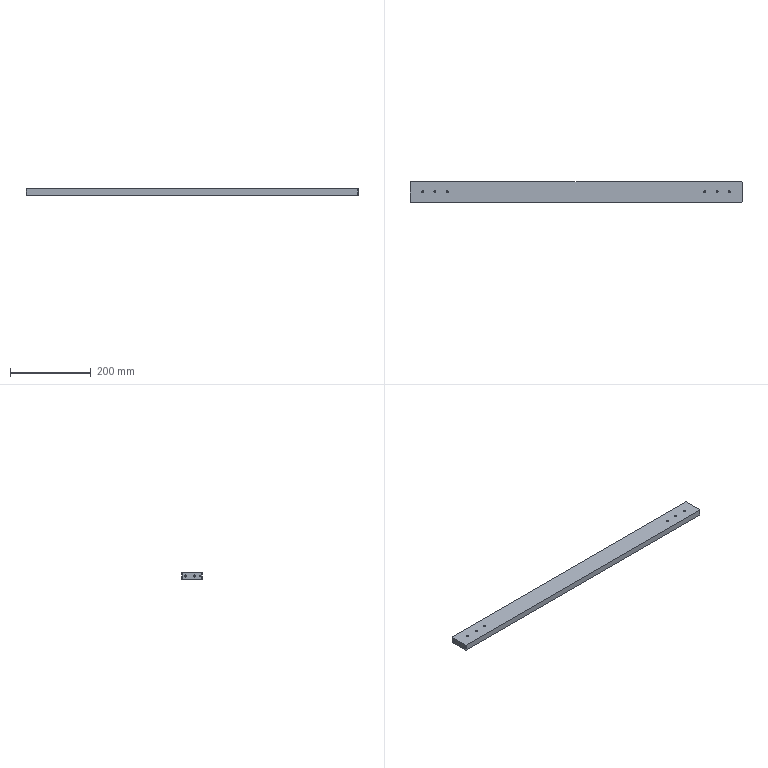Part | SolidWorks | features HoleWzd 3, Chamfer 1, Extrusion 1, MirrorPattern 1 | 1 solid | 46 faces | box 824 x 50 x 15 mm | volume 614536 mm3 | cylinder 24 | cone 12 | plane 10 | commonest cylinder face diameters 5 x20 3.3 x4
STEP:
#1=CARTESIAN_POINT('',(-29.5,25.,15.));
#2=VERTEX_POINT('',#1);
#3=CARTESIAN_POINT('',(-34.5,25.,15.));
#4=VERTEX_POINT('',#3);
#5=CARTESIAN_POINT('',(-32.,25.,15.));
#6=DIRECTION('',(0.,0.,-1.));
#7=DIRECTION('',(-1.,0.,0.));
#8=AXIS2_PLACEMENT_3D('',#5,#6,#7);
#9=CIRCLE('',#8,2.5);
#10=EDGE_CURVE('',#2,#4,#9,.T.);
#11=ORIENTED_EDGE('',*,*,#10,.F.);
#12=CARTESIAN_POINT('',(-29.5,25.,0.));
#13=VERTEX_POINT('',#12);
#14=CARTESIAN_POINT('',(-29.5,25.,0.));
#15=DIRECTION('',(0.,0.,-1.));
#16=VECTOR('',#15,1000.);
#17=LINE('',#14,#16);
#18=EDGE_CURVE('',#2,#13,#17,.T.);
#19=ORIENTED_EDGE('',*,*,#18,.T.);
#20=CARTESIAN_POINT('',(-34.5,25.,0.));
#21=VERTEX_POINT('',#20);
#22=CARTESIAN_POINT('',(-32.,25.,0.));
#23=DIRECTION('',(0.,0.,-1.));
#24=DIRECTION('',(-1.,0.,0.));
#25=AXIS2_PLACEMENT_3D('',#22,#23,#24);
#26=CIRCLE('',#25,2.5);
#27=EDGE_CURVE('',#13,#21,#26,.T.);
#28=ORIENTED_EDGE('',*,*,#27,.T.);
#29=CARTESIAN_POINT('',(-34.5,25.,0.));
#30=DIRECTION('',(0.,0.,-1.));
#31=VECTOR('',#30,1000.);
#32=LINE('',#29,#31);
#33=EDGE_CURVE('',#4,#21,#32,.T.);
#34=ORIENTED_EDGE('',*,*,#33,.F.);
#35=EDGE_LOOP('',(#11,#19,#28,#34));
#36=FACE_OUTER_BOUND('',#35,.T.);
#37=CARTESIAN_POINT('',(-32.,25.,0.));
#38=DIRECTION('',(0.,0.,-1.));
#39=DIRECTION('',(-1.,0.,0.));
#40=AXIS2_PLACEMENT_3D('',#37,#38,#39);
#41=CYLINDRICAL_SURFACE('',#40,2.5);
#42=ADVANCED_FACE('',(#36),#41,.F.);
#43=CARTESIAN_POINT('',(-59.5,25.,15.));
#44=VERTEX_POINT('',#43);
#45=CARTESIAN_POINT('',(-64.5,25.,15.));
#46=VERTEX_POINT('',#45);
#47=CARTESIAN_POINT('',(-62.,25.,15.));
#48=DIRECTION('',(0.,0.,-1.));
#49=DIRECTION('',(-1.,0.,0.));
#50=AXIS2_PLACEMENT_3D('',#47,#48,#49);
#51=CIRCLE('',#50,2.5);
#52=EDGE_CURVE('',#44,#46,#51,.T.);
#53=ORIENTED_EDGE('',*,*,#52,.F.);
#54=CARTESIAN_POINT('',(-59.5,25.,0.));
#55=VERTEX_POINT('',#54);
#56=CARTESIAN_POINT('',(-59.5,25.,0.));
#57=DIRECTION('',(0.,0.,-1.));
#58=VECTOR('',#57,1000.);
#59=LINE('',#56,#58);
#60=EDGE_CURVE('',#44,#55,#59,.T.);
#61=ORIENTED_EDGE('',*,*,#60,.T.);
#62=CARTESIAN_POINT('',(-64.5,25.,0.));
#63=VERTEX_POINT('',#62);
#64=CARTESIAN_POINT('',(-62.,25.,0.));
#65=DIRECTION('',(0.,0.,-1.));
#66=DIRECTION('',(-1.,0.,0.));
#67=AXIS2_PLACEMENT_3D('',#64,#65,#66);
#68=CIRCLE('',#67,2.5);
#69=EDGE_CURVE('',#55,#63,#68,.T.);
#70=ORIENTED_EDGE('',*,*,#69,.T.);
#71=CARTESIAN_POINT('',(-64.5,25.,0.));
#72=DIRECTION('',(0.,0.,-1.));
#73=VECTOR('',#72,1000.);
#74=LINE('',#71,#73);
#75=EDGE_CURVE('',#46,#63,#74,.T.);
#76=ORIENTED_EDGE('',*,*,#75,.F.);
#77=EDGE_LOOP('',(#53,#61,#70,#76));
#78=FACE_OUTER_BOUND('',#77,.T.);
#79=CARTESIAN_POINT('',(-62.,25.,0.));
#80=DIRECTION('',(0.,0.,-1.));
#81=DIRECTION('',(-1.,0.,0.));
#82=AXIS2_PLACEMENT_3D('',#79,#80,#81);
#83=CYLINDRICAL_SURFACE('',#82,2.5);
#84=ADVANCED_FACE('',(#78),#83,.F.);
#85=CARTESIAN_POINT('',(-89.5,25.,15.));
#86=VERTEX_POINT('',#85);
#87=CARTESIAN_POINT('',(-94.5,25.,15.));
#88=VERTEX_POINT('',#87);
#89=CARTESIAN_POINT('',(-92.,25.,15.));
#90=DIRECTION('',(0.,0.,-1.));
#91=DIRECTION('',(-1.,0.,0.));
#92=AXIS2_PLACEMENT_3D('',#89,#90,#91);
#93=CIRCLE('',#92,2.5);
#94=EDGE_CURVE('',#86,#88,#93,.T.);
#95=ORIENTED_EDGE('',*,*,#94,.F.);
#96=CARTESIAN_POINT('',(-89.5,25.,0.));
#97=VERTEX_POINT('',#96);
#98=CARTESIAN_POINT('',(-89.5,25.,0.));
#99=DIRECTION('',(0.,0.,-1.));
#100=VECTOR('',#99,1000.);
#101=LINE('',#98,#100);
#102=EDGE_CURVE('',#86,#97,#101,.T.);
#103=ORIENTED_EDGE('',*,*,#102,.T.);
#104=CARTESIAN_POINT('',(-94.5,25.,0.));
#105=VERTEX_POINT('',#104);
#106=CARTESIAN_POINT('',(-92.,25.,0.));
#107=DIRECTION('',(0.,0.,-1.));
#108=DIRECTION('',(-1.,0.,0.));
#109=AXIS2_PLACEMENT_3D('',#106,#107,#108);
#110=CIRCLE('',#109,2.5);
#111=EDGE_CURVE('',#97,#105,#110,.T.);
#112=ORIENTED_EDGE('',*,*,#111,.T.);
#113=CARTESIAN_POINT('',(-94.5,25.,0.));
#114=DIRECTION('',(0.,0.,-1.));
#115=VECTOR('',#114,1000.);
#116=LINE('',#113,#115);
#117=EDGE_CURVE('',#88,#105,#116,.T.);
#118=ORIENTED_EDGE('',*,*,#117,.F.);
#119=EDGE_LOOP('',(#95,#103,#112,#118));
#120=FACE_OUTER_BOUND('',#119,.T.);
#121=CARTESIAN_POINT('',(-92.,25.,0.));
#122=DIRECTION('',(0.,0.,-1.));
#123=DIRECTION('',(-1.,0.,0.));
#124=AXIS2_PLACEMENT_3D('',#121,#122,#123);
#125=CYLINDRICAL_SURFACE('',#124,2.5);
#126=ADVANCED_FACE('',(#120),#125,.F.);
#127=CARTESIAN_POINT('',(-729.5,25.,15.));
#128=VERTEX_POINT('',#127);
#129=CARTESIAN_POINT('',(-734.5,25.,15.));
#130=VERTEX_POINT('',#129);
#131=CARTESIAN_POINT('',(-732.,25.,15.));
#132=DIRECTION('',(0.,0.,-1.));
#133=DIRECTION('',(-1.,0.,0.));
#134=AXIS2_PLACEMENT_3D('',#131,#132,#133);
#135=CIRCLE('',#134,2.5);
#136=EDGE_CURVE('',#128,#130,#135,.T.);
#137=ORIENTED_EDGE('',*,*,#136,.F.);
#138=CARTESIAN_POINT('',(-729.5,25.,0.));
#139=VERTEX_POINT('',#138);
#140=CARTESIAN_POINT('',(-729.5,25.,0.));
#141=DIRECTION('',(0.,0.,-1.));
#142=VECTOR('',#141,1000.);
#143=LINE('',#140,#142);
#144=EDGE_CURVE('',#128,#139,#143,.T.);
#145=ORIENTED_EDGE('',*,*,#144,.T.);
#146=CARTESIAN_POINT('',(-734.5,25.,0.));
#147=VERTEX_POINT('',#146);
#148=CARTESIAN_POINT('',(-732.,25.,0.));
#149=DIRECTION('',(0.,0.,-1.));
#150=DIRECTION('',(-1.,0.,0.));
#151=AXIS2_PLACEMENT_3D('',#148,#149,#150);
#152=CIRCLE('',#151,2.5);
#153=EDGE_CURVE('',#139,#147,#152,.T.);
#154=ORIENTED_EDGE('',*,*,#153,.T.);
#155=CARTESIAN_POINT('',(-734.5,25.,0.));
#156=DIRECTION('',(0.,0.,-1.));
#157=VECTOR('',#156,1000.);
#158=LINE('',#155,#157);
#159=EDGE_CURVE('',#130,#147,#158,.T.);
#160=ORIENTED_EDGE('',*,*,#159,.F.);
#161=EDGE_LOOP('',(#137,#145,#154,#160));
#162=FACE_OUTER_BOUND('',#161,.T.);
#163=CARTESIAN_POINT('',(-732.,25.,0.));
#164=DIRECTION('',(0.,0.,-1.));
#165=DIRECTION('',(-1.,0.,0.));
#166=AXIS2_PLACEMENT_3D('',#163,#164,#165);
#167=CYLINDRICAL_SURFACE('',#166,2.5);
#168=ADVANCED_FACE('',(#162),#167,.F.);
#169=CARTESIAN_POINT('',(-759.5,25.,15.));
#170=VERTEX_POINT('',#169);
#171=CARTESIAN_POINT('',(-764.5,25.,15.));
#172=VERTEX_POINT('',#171);
#173=CARTESIAN_POINT('',(-762.,25.,15.));
#174=DIRECTION('',(0.,0.,-1.));
#175=DIRECTION('',(-1.,0.,0.));
#176=AXIS2_PLACEMENT_3D('',#173,#174,#175);
#177=CIRCLE('',#176,2.5);
#178=EDGE_CURVE('',#170,#172,#177,.T.);
#179=ORIENTED_EDGE('',*,*,#178,.F.);
#180=CARTESIAN_POINT('',(-759.5,25.,0.));
#181=VERTEX_POINT('',#180);
#182=CARTESIAN_POINT('',(-759.5,25.,0.));
#183=DIRECTION('',(0.,0.,-1.));
#184=VECTOR('',#183,1000.);
#185=LINE('',#182,#184);
#186=EDGE_CURVE('',#170,#181,#185,.T.);
#187=ORIENTED_EDGE('',*,*,#186,.T.);
#188=CARTESIAN_POINT('',(-764.5,25.,0.));
#189=VERTEX_POINT('',#188);
#190=CARTESIAN_POINT('',(-762.,25.,0.));
#191=DIRECTION('',(0.,0.,-1.));
#192=DIRECTION('',(-1.,0.,0.));
#193=AXIS2_PLACEMENT_3D('',#190,#191,#192);
#194=CIRCLE('',#193,2.5);
#195=EDGE_CURVE('',#181,#189,#194,.T.);
#196=ORIENTED_EDGE('',*,*,#195,.T.);
#197=CARTESIAN_POINT('',(-764.5,25.,0.));
#198=DIRECTION('',(0.,0.,-1.));
#199=VECTOR('',#198,1000.);
#200=LINE('',#197,#199);
#201=EDGE_CURVE('',#172,#189,#200,.T.);
#202=ORIENTED_EDGE('',*,*,#201,.F.);
#203=EDGE_LOOP('',(#179,#187,#196,#202));
#204=FACE_OUTER_BOUND('',#203,.T.);
#205=CARTESIAN_POINT('',(-762.,25.,0.));
#206=DIRECTION('',(0.,0.,-1.));
#207=DIRECTION('',(-1.,0.,0.));
#208=AXIS2_PLACEMENT_3D('',#205,#206,#207);
#209=CYLINDRICAL_SURFACE('',#208,2.5);
#210=ADVANCED_FACE('',(#204),#209,.F.);
#211=CARTESIAN_POINT('',(-789.5,25.,15.));
#212=VERTEX_POINT('',#211);
#213=CARTESIAN_POINT('',(-794.5,25.,15.));
#214=VERTEX_POINT('',#213);
#215=CARTESIAN_POINT('',(-792.,25.,15.));
#216=DIRECTION('',(0.,0.,-1.));
#217=DIRECTION('',(-1.,0.,0.));
#218=AXIS2_PLACEMENT_3D('',#215,#216,#217);
#219=CIRCLE('',#218,2.5);
#220=EDGE_CURVE('',#212,#214,#219,.T.);
#221=ORIENTED_EDGE('',*,*,#220,.F.);
#222=CARTESIAN_POINT('',(-789.5,25.,0.));
#223=VERTEX_POINT('',#222);
#224=CARTESIAN_POINT('',(-789.5,25.,0.));
#225=DIRECTION('',(0.,0.,-1.));
#226=VECTOR('',#225,1000.);
#227=LINE('',#224,#226);
#228=EDGE_CURVE('',#212,#223,#227,.T.);
#229=ORIENTED_EDGE('',*,*,#228,.T.);
#230=CARTESIAN_POINT('',(-794.5,25.,0.));
#231=VERTEX_POINT('',#230);
#232=CARTESIAN_POINT('',(-792.,25.,0.));
#233=DIRECTION('',(0.,0.,-1.));
#234=DIRECTION('',(-1.,0.,0.));
#235=AXIS2_PLACEMENT_3D('',#232,#233,#234);
#236=CIRCLE('',#235,2.5);
#237=EDGE_CURVE('',#223,#231,#236,.T.);
#238=ORIENTED_EDGE('',*,*,#237,.T.);
#239=CARTESIAN_POINT('',(-794.5,25.,0.));
#240=DIRECTION('',(0.,0.,-1.));
#241=VECTOR('',#240,1000.);
#242=LINE('',#239,#241);
#243=EDGE_CURVE('',#214,#231,#242,.T.);
#244=ORIENTED_EDGE('',*,*,#243,.F.);
#245=EDGE_LOOP('',(#221,#229,#238,#244));
#246=FACE_OUTER_BOUND('',#245,.T.);
#247=CARTESIAN_POINT('',(-792.,25.,0.));
#248=DIRECTION('',(0.,0.,-1.));
#249=DIRECTION('',(-1.,0.,0.));
#250=AXIS2_PLACEMENT_3D('',#247,#248,#249);
#251=CYLINDRICAL_SURFACE('',#250,2.5);
#252=ADVANCED_FACE('',(#246),#251,.F.);
#253=CARTESIAN_POINT('',(-812.5,5.,5.85));
#254=VERTEX_POINT('',#253);
#255=CARTESIAN_POINT('',(-812.5,5.,9.15));
#256=VERTEX_POINT('',#255);
#257=CARTESIAN_POINT('',(-812.5,5.,7.5));
#258=DIRECTION('',(-1.,0.,0.));
#259=DIRECTION('',(0.,0.,1.));
#260=AXIS2_PLACEMENT_3D('',#257,#258,#259);
#261=CIRCLE('',#260,1.65);
#262=EDGE_CURVE('',#254,#256,#261,.T.);
#263=ORIENTED_EDGE('',*,*,#262,.F.);
#264=CARTESIAN_POINT('',(-824.,5.,5.85));
#265=VERTEX_POINT('',#264);
#266=CARTESIAN_POINT('',(-824.,5.,5.85));
#267=DIRECTION('',(-1.,0.,0.));
#268=VECTOR('',#267,1000.);
#269=LINE('',#266,#268);
#270=EDGE_CURVE('',#254,#265,#269,.T.);
#271=ORIENTED_EDGE('',*,*,#270,.T.);
#272=CARTESIAN_POINT('',(-824.,5.,9.15));
#273=VERTEX_POINT('',#272);
#274=CARTESIAN_POINT('',(-824.,5.,7.5));
#275=DIRECTION('',(-1.,0.,0.));
#276=DIRECTION('',(0.,0.,1.));
#277=AXIS2_PLACEMENT_3D('',#274,#275,#276);
#278=CIRCLE('',#277,1.65);
#279=EDGE_CURVE('',#265,#273,#278,.T.);
#280=ORIENTED_EDGE('',*,*,#279,.T.);
#281=CARTESIAN_POINT('',(-824.,5.,9.15));
#282=DIRECTION('',(-1.,0.,0.));
#283=VECTOR('',#282,1000.);
#284=LINE('',#281,#283);
#285=EDGE_CURVE('',#256,#273,#284,.T.);
#286=ORIENTED_EDGE('',*,*,#285,.F.);
#287=EDGE_LOOP('',(#263,#271,#280,#286));
#288=FACE_OUTER_BOUND('',#287,.T.);
#289=CARTESIAN_POINT('',(-824.,5.,7.5));
#290=DIRECTION('',(-1.,0.,0.));
#291=DIRECTION('',(0.,0.,1.));
#292=AXIS2_PLACEMENT_3D('',#289,#290,#291);
#293=CYLINDRICAL_SURFACE('',#292,1.65);
#294=ADVANCED_FACE('',(#288),#293,.F.);
#295=CARTESIAN_POINT('',(-811.509,5.,7.5));
#296=VERTEX_POINT('',#295);
#297=CARTESIAN_POINT('',(-812.5,5.,9.15));
#298=DIRECTION('',(-0.515,0.,0.8572));
#299=VECTOR('',#298,1000.);
#300=LINE('',#297,#299);
#301=EDGE_CURVE('',#296,#256,#300,.T.);
#302=ORIENTED_EDGE('',*,*,#301,.F.);
#303=CARTESIAN_POINT('',(-812.5,5.,5.85));
#304=DIRECTION('',(-0.515,0.,-0.8572));
#305=VECTOR('',#304,1000.);
#306=LINE('',#303,#305);
#307=EDGE_CURVE('',#296,#254,#306,.T.);
#308=ORIENTED_EDGE('',*,*,#307,.T.);
#309=ORIENTED_EDGE('',*,*,#262,.T.);
#310=EDGE_LOOP('',(#302,#308,#309));
#311=FACE_OUTER_BOUND('',#310,.T.);
#312=CARTESIAN_POINT('',(-812.5,5.,7.5));
#313=DIRECTION('',(-1.,0.,0.));
#314=DIRECTION('',(0.,0.,1.));
#315=AXIS2_PLACEMENT_3D('',#312,#313,#314);
#316=CONICAL_SURFACE('',#315,1.65,1.03);
#317=ADVANCED_FACE('',(#311),#316,.F.);
#318=CARTESIAN_POINT('',(-807.,40.,5.));
#319=VERTEX_POINT('',#318);
#320=CARTESIAN_POINT('',(-807.,40.,10.));
#321=VERTEX_POINT('',#320);
#322=CARTESIAN_POINT('',(-807.,40.,7.5));
#323=DIRECTION('',(-1.,0.,0.));
#324=DIRECTION('',(0.,0.,1.));
#325=AXIS2_PLACEMENT_3D('',#322,#323,#324);
#326=CIRCLE('',#325,2.5);
#327=EDGE_CURVE('',#319,#321,#326,.T.);
#328=ORIENTED_EDGE('',*,*,#327,.F.);
#329=CARTESIAN_POINT('',(-824.,40.,5.));
#330=VERTEX_POINT('',#329);
#331=CARTESIAN_POINT('',(-824.,40.,5.));
#332=DIRECTION('',(-1.,0.,0.));
#333=VECTOR('',#332,1000.);
#334=LINE('',#331,#333);
#335=EDGE_CURVE('',#319,#330,#334,.T.);
#336=ORIENTED_EDGE('',*,*,#335,.T.);
#337=CARTESIAN_POINT('',(-824.,40.,10.));
#338=VERTEX_POINT('',#337);
#339=CARTESIAN_POINT('',(-824.,40.,7.5));
#340=DIRECTION('',(-1.,0.,0.));
#341=DIRECTION('',(0.,0.,1.));
#342=AXIS2_PLACEMENT_3D('',#339,#340,#341);
#343=CIRCLE('',#342,2.5);
#344=EDGE_CURVE('',#330,#338,#343,.T.);
#345=ORIENTED_EDGE('',*,*,#344,.T.);
#346=CARTESIAN_POINT('',(-824.,40.,10.));
#347=DIRECTION('',(-1.,0.,0.));
#348=VECTOR('',#347,1000.);
#349=LINE('',#346,#348);
#350=EDGE_CURVE('',#321,#338,#349,.T.);
#351=ORIENTED_EDGE('',*,*,#350,.F.);
#352=EDGE_LOOP('',(#328,#336,#345,#351));
#353=FACE_OUTER_BOUND('',#352,.T.);
#354=CARTESIAN_POINT('',(-824.,40.,7.5));
#355=DIRECTION('',(-1.,0.,0.));
#356=DIRECTION('',(0.,0.,1.));
#357=AXIS2_PLACEMENT_3D('',#354,#355,#356);
#358=CYLINDRICAL_SURFACE('',#357,2.5);
#359=ADVANCED_FACE('',(#353),#358,.F.);
#360=CARTESIAN_POINT('',(-805.498,40.,7.5));
#361=VERTEX_POINT('',#360);
#362=CARTESIAN_POINT('',(-807.,40.,10.));
#363=DIRECTION('',(-0.515,0.,0.8572));
#364=VECTOR('',#363,1000.);
#365=LINE('',#362,#364);
#366=EDGE_CURVE('',#361,#321,#365,.T.);
#367=ORIENTED_EDGE('',*,*,#366,.F.);
#368=CARTESIAN_POINT('',(-807.,40.,5.));
#369=DIRECTION('',(-0.515,0.,-0.8572));
#370=VECTOR('',#369,1000.);
#371=LINE('',#368,#370);
#372=EDGE_CURVE('',#361,#319,#371,.T.);
#373=ORIENTED_EDGE('',*,*,#372,.T.);
#374=ORIENTED_EDGE('',*,*,#327,.T.);
#375=EDGE_LOOP('',(#367,#373,#374));
#376=FACE_OUTER_BOUND('',#375,.T.);
#377=CARTESIAN_POINT('',(-807.,40.,7.5));
#378=DIRECTION('',(-1.,0.,0.));
#379=DIRECTION('',(0.,0.,1.));
#380=AXIS2_PLACEMENT_3D('',#377,#378,#379);
#381=CONICAL_SURFACE('',#380,2.5,1.03);
#382=ADVANCED_FACE('',(#376),#381,.F.);
#383=CARTESIAN_POINT('',(-807.,20.,5.));
#384=VERTEX_POINT('',#383);
#385=CARTESIAN_POINT('',(-807.,20.,10.));
#386=VERTEX_POINT('',#385);
#387=CARTESIAN_POINT('',(-807.,20.,7.5));
#388=DIRECTION('',(-1.,0.,0.));
#389=DIRECTION('',(0.,0.,1.));
#390=AXIS2_PLACEMENT_3D('',#387,#388,#389);
#391=CIRCLE('',#390,2.5);
#392=EDGE_CURVE('',#384,#386,#391,.T.);
#393=ORIENTED_EDGE('',*,*,#392,.F.);
#394=CARTESIAN_POINT('',(-824.,20.,5.));
#395=VERTEX_POINT('',#394);
#396=CARTESIAN_POINT('',(-824.,20.,5.));
#397=DIRECTION('',(-1.,0.,0.));
#398=VECTOR('',#397,1000.);
#399=LINE('',#396,#398);
#400=EDGE_CURVE('',#384,#395,#399,.T.);
#401=ORIENTED_EDGE('',*,*,#400,.T.);
#402=CARTESIAN_POINT('',(-824.,20.,10.));
#403=VERTEX_POINT('',#402);
#404=CARTESIAN_POINT('',(-824.,20.,7.5));
#405=DIRECTION('',(-1.,0.,0.));
#406=DIRECTION('',(0.,0.,1.));
#407=AXIS2_PLACEMENT_3D('',#404,#405,#406);
#408=CIRCLE('',#407,2.5);
#409=EDGE_CURVE('',#395,#403,#408,.T.);
#410=ORIENTED_EDGE('',*,*,#409,.T.);
#411=CARTESIAN_POINT('',(-824.,20.,10.));
#412=DIRECTION('',(-1.,0.,0.));
#413=VECTOR('',#412,1000.);
#414=LINE('',#411,#413);
#415=EDGE_CURVE('',#386,#403,#414,.T.);
#416=ORIENTED_EDGE('',*,*,#415,.F.);
#417=EDGE_LOOP('',(#393,#401,#410,#416));
#418=FACE_OUTER_BOUND('',#417,.T.);
#419=CARTESIAN_POINT('',(-824.,20.,7.5));
#420=DIRECTION('',(-1.,0.,0.));
#421=DIRECTION('',(0.,0.,1.));
#422=AXIS2_PLACEMENT_3D('',#419,#420,#421);
#423=CYLINDRICAL_SURFACE('',#422,2.5);
#424=ADVANCED_FACE('',(#418),#423,.F.);
#425=CARTESIAN_POINT('',(-805.498,20.,7.5));
#426=VERTEX_POINT('',#425);
#427=CARTESIAN_POINT('',(-807.,20.,10.));
#428=DIRECTION('',(-0.515,0.,0.8572));
#429=VECTOR('',#428,1000.);
#430=LINE('',#427,#429);
#431=EDGE_CURVE('',#426,#386,#430,.T.);
#432=ORIENTED_EDGE('',*,*,#431,.F.);
#433=CARTESIAN_POINT('',(-807.,20.,5.));
#434=DIRECTION('',(-0.515,0.,-0.8572));
#435=VECTOR('',#434,1000.);
#436=LINE('',#433,#435);
#437=EDGE_CURVE('',#426,#384,#436,.T.);
#438=ORIENTED_EDGE('',*,*,#437,.T.);
#439=ORIENTED_EDGE('',*,*,#392,.T.);
#440=EDGE_LOOP('',(#432,#438,#439));
#441=FACE_OUTER_BOUND('',#440,.T.);
#442=CARTESIAN_POINT('',(-807.,20.,7.5));
#443=DIRECTION('',(-1.,0.,0.));
#444=DIRECTION('',(0.,0.,1.));
#445=AXIS2_PLACEMENT_3D('',#442,#443,#444);
#446=CONICAL_SURFACE('',#445,2.5,1.03);
#447=ADVANCED_FACE('',(#441),#446,.F.);
#448=CARTESIAN_POINT('',(-11.5,5.,9.15));
#449=VERTEX_POINT('',#448);
#450=CARTESIAN_POINT('',(-11.5,5.,5.85));
#451=VERTEX_POINT('',#450);
#452=CARTESIAN_POINT('',(-11.5,5.,7.5));
#453=DIRECTION('',(1.,0.,0.));
#454=DIRECTION('',(0.,0.,-1.));
#455=AXIS2_PLACEMENT_3D('',#452,#453,#454);
#456=CIRCLE('',#455,1.65);
#457=EDGE_CURVE('',#449,#451,#456,.T.);
#458=ORIENTED_EDGE('',*,*,#457,.F.);
#459=CARTESIAN_POINT('',(0.,5.,9.15));
#460=VERTEX_POINT('',#459);
#461=CARTESIAN_POINT('',(0.,5.,9.15));
#462=DIRECTION('',(1.,0.,0.));
#463=VECTOR('',#462,1000.);
#464=LINE('',#461,#463);
#465=EDGE_CURVE('',#449,#460,#464,.T.);
#466=ORIENTED_EDGE('',*,*,#465,.T.);
#467=CARTESIAN_POINT('',(0.,5.,5.85));
#468=VERTEX_POINT('',#467);
#469=CARTESIAN_POINT('',(0.,5.,7.5));
#470=DIRECTION('',(1.,0.,0.));
#471=DIRECTION('',(0.,0.,-1.));
#472=AXIS2_PLACEMENT_3D('',#469,#470,#471);
#473=CIRCLE('',#472,1.65);
#474=EDGE_CURVE('',#460,#468,#473,.T.);
#475=ORIENTED_EDGE('',*,*,#474,.T.);
#476=CARTESIAN_POINT('',(0.,5.,5.85));
#477=DIRECTION('',(1.,0.,0.));
#478=VECTOR('',#477,1000.);
#479=LINE('',#476,#478);
#480=EDGE_CURVE('',#451,#468,#479,.T.);
#481=ORIENTED_EDGE('',*,*,#480,.F.);
#482=EDGE_LOOP('',(#458,#466,#475,#481));
#483=FACE_OUTER_BOUND('',#482,.T.);
#484=CARTESIAN_POINT('',(0.,5.,7.5));
#485=DIRECTION('',(1.,0.,0.));
#486=DIRECTION('',(0.,0.,-1.));
#487=AXIS2_PLACEMENT_3D('',#484,#485,#486);
#488=CYLINDRICAL_SURFACE('',#487,1.65);
#489=ADVANCED_FACE('',(#483),#488,.F.);
#490=CARTESIAN_POINT('',(-12.491,5.,7.5));
#491=VERTEX_POINT('',#490);
#492=CARTESIAN_POINT('',(-11.5,5.,5.85));
#493=DIRECTION('',(0.515,0.,-0.8572));
#494=VECTOR('',#493,1000.);
#495=LINE('',#492,#494);
#496=EDGE_CURVE('',#491,#451,#495,.T.);
#497=ORIENTED_EDGE('',*,*,#496,.F.);
#498=CARTESIAN_POINT('',(-11.5,5.,9.15));
#499=DIRECTION('',(0.515,0.,0.8572));
#500=VECTOR('',#499,1000.);
#501=LINE('',#498,#500);
#502=EDGE_CURVE('',#491,#449,#501,.T.);
#503=ORIENTED_EDGE('',*,*,#502,.T.);
#504=ORIENTED_EDGE('',*,*,#457,.T.);
#505=EDGE_LOOP('',(#497,#503,#504));
#506=FACE_OUTER_BOUND('',#505,.T.);
#507=CARTESIAN_POINT('',(-11.5,5.,7.5));
#508=DIRECTION('',(1.,0.,0.));
#509=DIRECTION('',(0.,0.,-1.));
#510=AXIS2_PLACEMENT_3D('',#507,#508,#509);
#511=CONICAL_SURFACE('',#510,1.65,1.03);
#512=ADVANCED_FACE('',(#506),#511,.F.);
#513=CARTESIAN_POINT('',(-17.,40.,10.));
#514=VERTEX_POINT('',#513);
#515=CARTESIAN_POINT('',(-17.,40.,5.));
#516=VERTEX_POINT('',#515);
#517=CARTESIAN_POINT('',(-17.,40.,7.5));
#518=DIRECTION('',(1.,0.,0.));
#519=DIRECTION('',(0.,0.,-1.));
#520=AXIS2_PLACEMENT_3D('',#517,#518,#519);
#521=CIRCLE('',#520,2.5);
#522=EDGE_CURVE('',#514,#516,#521,.T.);
#523=ORIENTED_EDGE('',*,*,#522,.F.);
#524=CARTESIAN_POINT('',(0.,40.,10.));
#525=VERTEX_POINT('',#524);
#526=CARTESIAN_POINT('',(0.,40.,10.));
#527=DIRECTION('',(1.,0.,0.));
#528=VECTOR('',#527,1000.);
#529=LINE('',#526,#528);
#530=EDGE_CURVE('',#514,#525,#529,.T.);
#531=ORIENTED_EDGE('',*,*,#530,.T.);
#532=CARTESIAN_POINT('',(0.,40.,5.));
#533=VERTEX_POINT('',#532);
#534=CARTESIAN_POINT('',(0.,40.,7.5));
#535=DIRECTION('',(1.,0.,0.));
#536=DIRECTION('',(0.,0.,-1.));
#537=AXIS2_PLACEMENT_3D('',#534,#535,#536);
#538=CIRCLE('',#537,2.5);
#539=EDGE_CURVE('',#525,#533,#538,.T.);
#540=ORIENTED_EDGE('',*,*,#539,.T.);
#541=CARTESIAN_POINT('',(0.,40.,5.));
#542=DIRECTION('',(1.,0.,0.));
#543=VECTOR('',#542,1000.);
#544=LINE('',#541,#543);
#545=EDGE_CURVE('',#516,#533,#544,.T.);
#546=ORIENTED_EDGE('',*,*,#545,.F.);
#547=EDGE_LOOP('',(#523,#531,#540,#546));
#548=FACE_OUTER_BOUND('',#547,.T.);
#549=CARTESIAN_POINT('',(0.,40.,7.5));
#550=DIRECTION('',(1.,0.,0.));
#551=DIRECTION('',(0.,0.,-1.));
#552=AXIS2_PLACEMENT_3D('',#549,#550,#551);
#553=CYLINDRICAL_SURFACE('',#552,2.5);
#554=ADVANCED_FACE('',(#548),#553,.F.);
#555=CARTESIAN_POINT('',(-18.502,40.,7.5));
#556=VERTEX_POINT('',#555);
#557=CARTESIAN_POINT('',(-17.,40.,5.));
#558=DIRECTION('',(0.515,0.,-0.8572));
#559=VECTOR('',#558,1000.);
#560=LINE('',#557,#559);
#561=EDGE_CURVE('',#556,#516,#560,.T.);
#562=ORIENTED_EDGE('',*,*,#561,.F.);
#563=CARTESIAN_POINT('',(-17.,40.,10.));
#564=DIRECTION('',(0.515,0.,0.8572));
#565=VECTOR('',#564,1000.);
#566=LINE('',#563,#565);
#567=EDGE_CURVE('',#556,#514,#566,.T.);
#568=ORIENTED_EDGE('',*,*,#567,.T.);
#569=ORIENTED_EDGE('',*,*,#522,.T.);
#570=EDGE_LOOP('',(#562,#568,#569));
#571=FACE_OUTER_BOUND('',#570,.T.);
#572=CARTESIAN_POINT('',(-17.,40.,7.5));
#573=DIRECTION('',(1.,0.,0.));
#574=DIRECTION('',(0.,0.,-1.));
#575=AXIS2_PLACEMENT_3D('',#572,#573,#574);
#576=CONICAL_SURFACE('',#575,2.5,1.03);
#577=ADVANCED_FACE('',(#571),#576,.F.);
#578=CARTESIAN_POINT('',(-17.,20.,10.));
#579=VERTEX_POINT('',#578);
#580=CARTESIAN_POINT('',(-17.,20.,5.));
#581=VERTEX_POINT('',#580);
#582=CARTESIAN_POINT('',(-17.,20.,7.5));
#583=DIRECTION('',(1.,0.,0.));
#584=DIRECTION('',(0.,0.,-1.));
#585=AXIS2_PLACEMENT_3D('',#582,#583,#584);
#586=CIRCLE('',#585,2.5);
#587=EDGE_CURVE('',#579,#581,#586,.T.);
#588=ORIENTED_EDGE('',*,*,#587,.F.);
#589=CARTESIAN_POINT('',(0.,20.,10.));
#590=VERTEX_POINT('',#589);
#591=CARTESIAN_POINT('',(0.,20.,10.));
#592=DIRECTION('',(1.,0.,0.));
#593=VECTOR('',#592,1000.);
#594=LINE('',#591,#593);
#595=EDGE_CURVE('',#579,#590,#594,.T.);
#596=ORIENTED_EDGE('',*,*,#595,.T.);
#597=CARTESIAN_POINT('',(0.,20.,5.));
#598=VERTEX_POINT('',#597);
#599=CARTESIAN_POINT('',(0.,20.,7.5));
#600=DIRECTION('',(1.,0.,0.));
#601=DIRECTION('',(0.,0.,-1.));
#602=AXIS2_PLACEMENT_3D('',#599,#600,#601);
#603=CIRCLE('',#602,2.5);
#604=EDGE_CURVE('',#590,#598,#603,.T.);
#605=ORIENTED_EDGE('',*,*,#604,.T.);
#606=CARTESIAN_POINT('',(0.,20.,5.));
#607=DIRECTION('',(1.,0.,0.));
#608=VECTOR('',#607,1000.);
#609=LINE('',#606,#608);
#610=EDGE_CURVE('',#581,#598,#609,.T.);
#611=ORIENTED_EDGE('',*,*,#610,.F.);
#612=EDGE_LOOP('',(#588,#596,#605,#611));
#613=FACE_OUTER_BOUND('',#612,.T.);
#614=CARTESIAN_POINT('',(0.,20.,7.5));
#615=DIRECTION('',(1.,0.,0.));
#616=DIRECTION('',(0.,0.,-1.));
#617=AXIS2_PLACEMENT_3D('',#614,#615,#616);
#618=CYLINDRICAL_SURFACE('',#617,2.5);
#619=ADVANCED_FACE('',(#613),#618,.F.);
#620=CARTESIAN_POINT('',(-18.502,20.,7.5));
#621=VERTEX_POINT('',#620);
#622=CARTESIAN_POINT('',(-17.,20.,5.));
#623=DIRECTION('',(0.515,0.,-0.8572));
#624=VECTOR('',#623,1000.);
#625=LINE('',#622,#624);
#626=EDGE_CURVE('',#621,#581,#625,.T.);
#627=ORIENTED_EDGE('',*,*,#626,.F.);
#628=CARTESIAN_POINT('',(-17.,20.,10.));
#629=DIRECTION('',(0.515,0.,0.8572));
#630=VECTOR('',#629,1000.);
#631=LINE('',#628,#630);
#632=EDGE_CURVE('',#621,#579,#631,.T.);
#633=ORIENTED_EDGE('',*,*,#632,.T.);
#634=ORIENTED_EDGE('',*,*,#587,.T.);
#635=EDGE_LOOP('',(#627,#633,#634));
#636=FACE_OUTER_BOUND('',#635,.T.);
#637=CARTESIAN_POINT('',(-17.,20.,7.5));
#638=DIRECTION('',(1.,0.,0.));
#639=DIRECTION('',(0.,0.,-1.));
#640=AXIS2_PLACEMENT_3D('',#637,#638,#639);
#641=CONICAL_SURFACE('',#640,2.5,1.03);
#642=ADVANCED_FACE('',(#636),#641,.F.);
#643=CARTESIAN_POINT('',(-2.,50.,0.));
#644=VERTEX_POINT('',#643);
#645=CARTESIAN_POINT('',(-822.,50.,0.));
#646=VERTEX_POINT('',#645);
#647=CARTESIAN_POINT('',(-824.,50.,0.));
#648=DIRECTION('',(-1.,0.,0.));
#649=VECTOR('',#648,1000.);
#650=LINE('',#647,#649);
#651=EDGE_CURVE('',#644,#646,#650,.T.);
#652=ORIENTED_EDGE('',*,*,#651,.T.);
#653=CARTESIAN_POINT('',(-822.,50.,15.));
#654=VERTEX_POINT('',#653);
#655=CARTESIAN_POINT('',(-822.,50.,15.));
#656=DIRECTION('',(0.,0.,1.));
#657=VECTOR('',#656,1000.);
#658=LINE('',#655,#657);
#659=EDGE_CURVE('',#646,#654,#658,.T.);
#660=ORIENTED_EDGE('',*,*,#659,.T.);
#661=CARTESIAN_POINT('',(-2.,50.,15.));
#662=VERTEX_POINT('',#661);
#663=CARTESIAN_POINT('',(-824.,50.,15.));
#664=DIRECTION('',(-1.,0.,0.));
#665=VECTOR('',#664,1000.);
#666=LINE('',#663,#665);
#667=EDGE_CURVE('',#662,#654,#666,.T.);
#668=ORIENTED_EDGE('',*,*,#667,.F.);
#669=CARTESIAN_POINT('',(-2.,50.,15.));
#670=DIRECTION('',(0.,0.,-1.));
#671=VECTOR('',#670,1000.);
#672=LINE('',#669,#671);
#673=EDGE_CURVE('',#662,#644,#672,.T.);
#674=ORIENTED_EDGE('',*,*,#673,.T.);
#675=EDGE_LOOP('',(#652,#660,#668,#674));
#676=FACE_OUTER_BOUND('',#675,.T.);
#677=CARTESIAN_POINT('',(-824.,50.,15.));
#678=DIRECTION('',(0.,-1.,0.));
#679=DIRECTION('',(1.,0.,0.));
#680=AXIS2_PLACEMENT_3D('',#677,#678,#679);
#681=PLANE('',#680);
#682=ADVANCED_FACE('',(#676),#681,.F.);
#683=CARTESIAN_POINT('',(-824.,5.,7.5));
#684=DIRECTION('',(-1.,0.,0.));
#685=DIRECTION('',(0.,0.,1.));
#686=AXIS2_PLACEMENT_3D('',#683,#684,#685);
#687=CIRCLE('',#686,1.65);
#688=EDGE_CURVE('',#273,#265,#687,.T.);
#689=ORIENTED_EDGE('',*,*,#688,.F.);
#690=ORIENTED_EDGE('',*,*,#279,.F.);
#691=EDGE_LOOP('',(#689,#690));
#692=FACE_BOUND('',#691,.T.);
#693=CARTESIAN_POINT('',(-824.,40.,7.5));
#694=DIRECTION('',(-1.,0.,0.));
#695=DIRECTION('',(0.,0.,1.));
#696=AXIS2_PLACEMENT_3D('',#693,#694,#695);
#697=CIRCLE('',#696,2.5);
#698=EDGE_CURVE('',#338,#330,#697,.T.);
#699=ORIENTED_EDGE('',*,*,#698,.F.);
#700=ORIENTED_EDGE('',*,*,#344,.F.);
#701=EDGE_LOOP('',(#699,#700));
#702=FACE_BOUND('',#701,.T.);
#703=CARTESIAN_POINT('',(-824.,20.,7.5));
#704=DIRECTION('',(-1.,0.,0.));
#705=DIRECTION('',(0.,0.,1.));
#706=AXIS2_PLACEMENT_3D('',#703,#704,#705);
#707=CIRCLE('',#706,2.5);
#708=EDGE_CURVE('',#403,#395,#707,.T.);
#709=ORIENTED_EDGE('',*,*,#708,.F.);
#710=ORIENTED_EDGE('',*,*,#409,.F.);
#711=EDGE_LOOP('',(#709,#710));
#712=FACE_BOUND('',#711,.T.);
#713=CARTESIAN_POINT('',(-824.,48.,15.));
#714=VERTEX_POINT('',#713);
#715=CARTESIAN_POINT('',(-824.,2.,15.));
#716=VERTEX_POINT('',#715);
#717=CARTESIAN_POINT('',(-824.,50.,15.));
#718=DIRECTION('',(0.,-1.,0.));
#719=VECTOR('',#718,1000.);
#720=LINE('',#717,#719);
#721=EDGE_CURVE('',#714,#716,#720,.T.);
#722=ORIENTED_EDGE('',*,*,#721,.F.);
#723=CARTESIAN_POINT('',(-824.,48.,0.));
#724=VERTEX_POINT('',#723);
#725=CARTESIAN_POINT('',(-824.,48.,15.));
#726=DIRECTION('',(0.,0.,-1.));
#727=VECTOR('',#726,1000.);
#728=LINE('',#725,#727);
#729=EDGE_CURVE('',#714,#724,#728,.T.);
#730=ORIENTED_EDGE('',*,*,#729,.T.);
#731=CARTESIAN_POINT('',(-824.,2.,0.));
#732=VERTEX_POINT('',#731);
#733=CARTESIAN_POINT('',(-824.,50.,0.));
#734=DIRECTION('',(0.,-1.,0.));
#735=VECTOR('',#734,1000.);
#736=LINE('',#733,#735);
#737=EDGE_CURVE('',#724,#732,#736,.T.);
#738=ORIENTED_EDGE('',*,*,#737,.T.);
#739=CARTESIAN_POINT('',(-824.,2.,15.));
#740=DIRECTION('',(0.,0.,1.));
#741=VECTOR('',#740,1000.);
#742=LINE('',#739,#741);
#743=EDGE_CURVE('',#732,#716,#742,.T.);
#744=ORIENTED_EDGE('',*,*,#743,.T.);
#745=EDGE_LOOP('',(#722,#730,#738,#744));
#746=FACE_OUTER_BOUND('',#745,.T.);
#747=CARTESIAN_POINT('',(-824.,50.,15.));
#748=DIRECTION('',(1.,0.,0.));
#749=DIRECTION('',(0.,1.,0.));
#750=AXIS2_PLACEMENT_3D('',#747,#748,#749);
#751=PLANE('',#750);
#752=ADVANCED_FACE('',(#692,#702,#712,#746),#751,.F.);
#753=CARTESIAN_POINT('',(-822.,0.,15.));
#754=VERTEX_POINT('',#753);
#755=CARTESIAN_POINT('',(-2.,0.,15.));
#756=VERTEX_POINT('',#755);
#757=CARTESIAN_POINT('',(-824.,0.,15.));
#758=DIRECTION('',(1.,0.,0.));
#759=VECTOR('',#758,1000.);
#760=LINE('',#757,#759);
#761=EDGE_CURVE('',#754,#756,#760,.T.);
#762=ORIENTED_EDGE('',*,*,#761,.F.);
#763=CARTESIAN_POINT('',(-822.,0.,0.));
#764=VERTEX_POINT('',#763);
#765=CARTESIAN_POINT('',(-822.,0.,15.));
#766=DIRECTION('',(0.,0.,-1.));
#767=VECTOR('',#766,1000.);
#768=LINE('',#765,#767);
#769=EDGE_CURVE('',#754,#764,#768,.T.);
#770=ORIENTED_EDGE('',*,*,#769,.T.);
#771=CARTESIAN_POINT('',(-2.,0.,0.));
#772=VERTEX_POINT('',#771);
#773=CARTESIAN_POINT('',(-824.,0.,0.));
#774=DIRECTION('',(1.,0.,0.));
#775=VECTOR('',#774,1000.);
#776=LINE('',#773,#775);
#777=EDGE_CURVE('',#764,#772,#776,.T.);
#778=ORIENTED_EDGE('',*,*,#777,.T.);
#779=CARTESIAN_POINT('',(-2.,0.,15.));
#780=DIRECTION('',(0.,0.,1.));
#781=VECTOR('',#780,1000.);
#782=LINE('',#779,#781);
#783=EDGE_CURVE('',#772,#756,#782,.T.);
#784=ORIENTED_EDGE('',*,*,#783,.T.);
#785=EDGE_LOOP('',(#762,#770,#778,#784));
#786=FACE_OUTER_BOUND('',#785,.T.);
#787=CARTESIAN_POINT('',(-824.,0.,15.));
#788=DIRECTION('',(0.,1.,0.));
#789=DIRECTION('',(0.,0.,1.));
#790=AXIS2_PLACEMENT_3D('',#787,#788,#789);
#791=PLANE('',#790);
#792=ADVANCED_FACE('',(#786),#791,.F.);
#793=CARTESIAN_POINT('',(0.,5.,7.5));
#794=DIRECTION('',(1.,0.,0.));
#795=DIRECTION('',(0.,0.,-1.));
#796=AXIS2_PLACEMENT_3D('',#793,#794,#795);
#797=CIRCLE('',#796,1.65);
#798=EDGE_CURVE('',#468,#460,#797,.T.);
#799=ORIENTED_EDGE('',*,*,#798,.F.);
#800=ORIENTED_EDGE('',*,*,#474,.F.);
#801=EDGE_LOOP('',(#799,#800));
#802=FACE_BOUND('',#801,.T.);
#803=CARTESIAN_POINT('',(0.,40.,7.5));
#804=DIRECTION('',(1.,0.,0.));
#805=DIRECTION('',(0.,0.,-1.));
#806=AXIS2_PLACEMENT_3D('',#803,#804,#805);
#807=CIRCLE('',#806,2.5);
#808=EDGE_CURVE('',#533,#525,#807,.T.);
#809=ORIENTED_EDGE('',*,*,#808,.F.);
#810=ORIENTED_EDGE('',*,*,#539,.F.);
#811=EDGE_LOOP('',(#809,#810));
#812=FACE_BOUND('',#811,.T.);
#813=CARTESIAN_POINT('',(0.,20.,7.5));
#814=DIRECTION('',(1.,0.,0.));
#815=DIRECTION('',(0.,0.,-1.));
#816=AXIS2_PLACEMENT_3D('',#813,#814,#815);
#817=CIRCLE('',#816,2.5);
#818=EDGE_CURVE('',#598,#590,#817,.T.);
#819=ORIENTED_EDGE('',*,*,#818,.F.);
#820=ORIENTED_EDGE('',*,*,#604,.F.);
#821=EDGE_LOOP('',(#819,#820));
#822=FACE_BOUND('',#821,.T.);
#823=CARTESIAN_POINT('',(0.,2.,0.));
#824=VERTEX_POINT('',#823);
#825=CARTESIAN_POINT('',(0.,48.,0.));
#826=VERTEX_POINT('',#825);
#827=CARTESIAN_POINT('',(0.,50.,0.));
#828=DIRECTION('',(0.,1.,0.));
#829=VECTOR('',#828,1000.);
#830=LINE('',#827,#829);
#831=EDGE_CURVE('',#824,#826,#830,.T.);
#832=ORIENTED_EDGE('',*,*,#831,.T.);
#833=CARTESIAN_POINT('',(0.,48.,15.));
#834=VERTEX_POINT('',#833);
#835=CARTESIAN_POINT('',(0.,48.,15.));
#836=DIRECTION('',(0.,0.,1.));
#837=VECTOR('',#836,1000.);
#838=LINE('',#835,#837);
#839=EDGE_CURVE('',#826,#834,#838,.T.);
#840=ORIENTED_EDGE('',*,*,#839,.T.);
#841=CARTESIAN_POINT('',(0.,2.,15.));
#842=VERTEX_POINT('',#841);
#843=CARTESIAN_POINT('',(0.,50.,15.));
#844=DIRECTION('',(0.,1.,0.));
#845=VECTOR('',#844,1000.);
#846=LINE('',#843,#845);
#847=EDGE_CURVE('',#842,#834,#846,.T.);
#848=ORIENTED_EDGE('',*,*,#847,.F.);
#849=CARTESIAN_POINT('',(0.,2.,15.));
#850=DIRECTION('',(0.,0.,-1.));
#851=VECTOR('',#850,1000.);
#852=LINE('',#849,#851);
#853=EDGE_CURVE('',#842,#824,#852,.T.);
#854=ORIENTED_EDGE('',*,*,#853,.T.);
#855=EDGE_LOOP('',(#832,#840,#848,#854));
#856=FACE_OUTER_BOUND('',#855,.T.);
#857=CARTESIAN_POINT('',(0.,50.,15.));
#858=DIRECTION('',(-1.,0.,0.));
#859=DIRECTION('',(0.,-1.,0.));
#860=AXIS2_PLACEMENT_3D('',#857,#858,#859);
#861=PLANE('',#860);
#862=ADVANCED_FACE('',(#802,#812,#822,#856),#861,.F.);
#863=CARTESIAN_POINT('',(-32.,25.,15.));
#864=DIRECTION('',(0.,0.,-1.));
#865=DIRECTION('',(-1.,0.,0.));
#866=AXIS2_PLACEMENT_3D('',#863,#864,#865);
#867=CIRCLE('',#866,2.5);
#868=EDGE_CURVE('',#4,#2,#867,.T.);
#869=ORIENTED_EDGE('',*,*,#868,.T.);
#870=ORIENTED_EDGE('',*,*,#10,.T.);
#871=EDGE_LOOP('',(#869,#870));
#872=FACE_BOUND('',#871,.T.);
#873=CARTESIAN_POINT('',(-62.,25.,15.));
#874=DIRECTION('',(0.,0.,-1.));
#875=DIRECTION('',(-1.,0.,0.));
#876=AXIS2_PLACEMENT_3D('',#873,#874,#875);
#877=CIRCLE('',#876,2.5);
#878=EDGE_CURVE('',#46,#44,#877,.T.);
#879=ORIENTED_EDGE('',*,*,#878,.T.);
#880=ORIENTED_EDGE('',*,*,#52,.T.);
#881=EDGE_LOOP('',(#879,#880));
#882=FACE_BOUND('',#881,.T.);
#883=CARTESIAN_POINT('',(-92.,25.,15.));
#884=DIRECTION('',(0.,0.,-1.));
#885=DIRECTION('',(-1.,0.,0.));
#886=AXIS2_PLACEMENT_3D('',#883,#884,#885);
#887=CIRCLE('',#886,2.5);
#888=EDGE_CURVE('',#88,#86,#887,.T.);
#889=ORIENTED_EDGE('',*,*,#888,.T.);
#890=ORIENTED_EDGE('',*,*,#94,.T.);
#891=EDGE_LOOP('',(#889,#890));
#892=FACE_BOUND('',#891,.T.);
#893=CARTESIAN_POINT('',(-732.,25.,15.));
#894=DIRECTION('',(0.,0.,-1.));
#895=DIRECTION('',(-1.,0.,0.));
#896=AXIS2_PLACEMENT_3D('',#893,#894,#895);
#897=CIRCLE('',#896,2.5);
#898=EDGE_CURVE('',#130,#128,#897,.T.);
#899=ORIENTED_EDGE('',*,*,#898,.T.);
#900=ORIENTED_EDGE('',*,*,#136,.T.);
#901=EDGE_LOOP('',(#899,#900));
#902=FACE_BOUND('',#901,.T.);
#903=CARTESIAN_POINT('',(-762.,25.,15.));
#904=DIRECTION('',(0.,0.,-1.));
#905=DIRECTION('',(-1.,0.,0.));
#906=AXIS2_PLACEMENT_3D('',#903,#904,#905);
#907=CIRCLE('',#906,2.5);
#908=EDGE_CURVE('',#172,#170,#907,.T.);
#909=ORIENTED_EDGE('',*,*,#908,.T.);
#910=ORIENTED_EDGE('',*,*,#178,.T.);
#911=EDGE_LOOP('',(#909,#910));
#912=FACE_BOUND('',#911,.T.);
#913=CARTESIAN_POINT('',(-792.,25.,15.));
#914=DIRECTION('',(0.,0.,-1.));
#915=DIRECTION('',(-1.,0.,0.));
#916=AXIS2_PLACEMENT_3D('',#913,#914,#915);
#917=CIRCLE('',#916,2.5);
#918=EDGE_CURVE('',#214,#212,#917,.T.);
#919=ORIENTED_EDGE('',*,*,#918,.T.);
#920=ORIENTED_EDGE('',*,*,#220,.T.);
#921=EDGE_LOOP('',(#919,#920));
#922=FACE_BOUND('',#921,.T.);
#923=ORIENTED_EDGE('',*,*,#667,.T.);
#924=CARTESIAN_POINT('',(-824.,48.,15.));
#925=DIRECTION('',(-0.7071,-0.7071,0.));
#926=VECTOR('',#925,1000.);
#927=LINE('',#924,#926);
#928=EDGE_CURVE('',#654,#714,#927,.T.);
#929=ORIENTED_EDGE('',*,*,#928,.T.);
#930=ORIENTED_EDGE('',*,*,#721,.T.);
#931=CARTESIAN_POINT('',(-822.,0.,15.));
#932=DIRECTION('',(0.7071,-0.7071,0.));
#933=VECTOR('',#932,1000.);
#934=LINE('',#931,#933);
#935=EDGE_CURVE('',#716,#754,#934,.T.);
#936=ORIENTED_EDGE('',*,*,#935,.T.);
#937=ORIENTED_EDGE('',*,*,#761,.T.);
#938=CARTESIAN_POINT('',(0.,2.,15.));
#939=DIRECTION('',(0.7071,0.7071,0.));
#940=VECTOR('',#939,1000.);
#941=LINE('',#938,#940);
#942=EDGE_CURVE('',#756,#842,#941,.T.);
#943=ORIENTED_EDGE('',*,*,#942,.T.);
#944=ORIENTED_EDGE('',*,*,#847,.T.);
#945=CARTESIAN_POINT('',(-2.,50.,15.));
#946=DIRECTION('',(-0.7071,0.7071,0.));
#947=VECTOR('',#946,1000.);
#948=LINE('',#945,#947);
#949=EDGE_CURVE('',#834,#662,#948,.T.);
#950=ORIENTED_EDGE('',*,*,#949,.T.);
#951=EDGE_LOOP('',(#923,#929,#930,#936,#937,#943,#944,#950));
#952=FACE_OUTER_BOUND('',#951,.T.);
#953=CARTESIAN_POINT('',(0.,0.,15.));
#954=DIRECTION('',(0.,0.,-1.));
#955=DIRECTION('',(-1.,0.,0.));
#956=AXIS2_PLACEMENT_3D('',#953,#954,#955);
#957=PLANE('',#956);
#958=ADVANCED_FACE('',(#872,#882,#892,#902,#912,#922,#952),#957,.F.);
#959=CARTESIAN_POINT('',(-32.,25.,0.));
#960=DIRECTION('',(0.,0.,-1.));
#961=DIRECTION('',(-1.,0.,0.));
#962=AXIS2_PLACEMENT_3D('',#959,#960,#961);
#963=CIRCLE('',#962,2.5);
#964=EDGE_CURVE('',#21,#13,#963,.T.);
#965=ORIENTED_EDGE('',*,*,#964,.F.);
#966=ORIENTED_EDGE('',*,*,#27,.F.);
#967=EDGE_LOOP('',(#965,#966));
#968=FACE_BOUND('',#967,.T.);
#969=CARTESIAN_POINT('',(-62.,25.,0.));
#970=DIRECTION('',(0.,0.,-1.));
#971=DIRECTION('',(-1.,0.,0.));
#972=AXIS2_PLACEMENT_3D('',#969,#970,#971);
#973=CIRCLE('',#972,2.5);
#974=EDGE_CURVE('',#63,#55,#973,.T.);
#975=ORIENTED_EDGE('',*,*,#974,.F.);
#976=ORIENTED_EDGE('',*,*,#69,.F.);
#977=EDGE_LOOP('',(#975,#976));
#978=FACE_BOUND('',#977,.T.);
#979=CARTESIAN_POINT('',(-92.,25.,0.));
#980=DIRECTION('',(0.,0.,-1.));
#981=DIRECTION('',(-1.,0.,0.));
#982=AXIS2_PLACEMENT_3D('',#979,#980,#981);
#983=CIRCLE('',#982,2.5);
#984=EDGE_CURVE('',#105,#97,#983,.T.);
#985=ORIENTED_EDGE('',*,*,#984,.F.);
#986=ORIENTED_EDGE('',*,*,#111,.F.);
#987=EDGE_LOOP('',(#985,#986));
#988=FACE_BOUND('',#987,.T.);
#989=CARTESIAN_POINT('',(-732.,25.,0.));
#990=DIRECTION('',(0.,0.,-1.));
#991=DIRECTION('',(-1.,0.,0.));
#992=AXIS2_PLACEMENT_3D('',#989,#990,#991);
#993=CIRCLE('',#992,2.5);
#994=EDGE_CURVE('',#147,#139,#993,.T.);
#995=ORIENTED_EDGE('',*,*,#994,.F.);
#996=ORIENTED_EDGE('',*,*,#153,.F.);
#997=EDGE_LOOP('',(#995,#996));
#998=FACE_BOUND('',#997,.T.);
#999=CARTESIAN_POINT('',(-762.,25.,0.));
#1000=DIRECTION('',(0.,0.,-1.));
#1001=DIRECTION('',(-1.,0.,0.));
#1002=AXIS2_PLACEMENT_3D('',#999,#1000,#1001);
#1003=CIRCLE('',#1002,2.5);
#1004=EDGE_CURVE('',#189,#181,#1003,.T.);
#1005=ORIENTED_EDGE('',*,*,#1004,.F.);
#1006=ORIENTED_EDGE('',*,*,#195,.F.);
#1007=EDGE_LOOP('',(#1005,#1006));
#1008=FACE_BOUND('',#1007,.T.);
#1009=CARTESIAN_POINT('',(-792.,25.,0.));
#1010=DIRECTION('',(0.,0.,-1.));
#1011=DIRECTION('',(-1.,0.,0.));
#1012=AXIS2_PLACEMENT_3D('',#1009,#1010,#1011);
#1013=CIRCLE('',#1012,2.5);
#1014=EDGE_CURVE('',#231,#223,#1013,.T.);
#1015=ORIENTED_EDGE('',*,*,#1014,.F.);
#1016=ORIENTED_EDGE('',*,*,#237,.F.);
#1017=EDGE_LOOP('',(#1015,#1016));
#1018=FACE_BOUND('',#1017,.T.);
#1019=ORIENTED_EDGE('',*,*,#737,.F.);
#1020=CARTESIAN_POINT('',(-436.,436.,0.));
#1021=DIRECTION('',(0.7071,0.7071,0.));
#1022=VECTOR('',#1021,1000.);
#1023=LINE('',#1020,#1022);
#1024=EDGE_CURVE('',#724,#646,#1023,.T.);
#1025=ORIENTED_EDGE('',*,*,#1024,.T.);
#1026=ORIENTED_EDGE('',*,*,#651,.F.);
#1027=CARTESIAN_POINT('',(24.,24.,0.));
#1028=DIRECTION('',(0.7071,-0.7071,0.));
#1029=VECTOR('',#1028,1000.);
#1030=LINE('',#1027,#1029);
#1031=EDGE_CURVE('',#644,#826,#1030,.T.);
#1032=ORIENTED_EDGE('',*,*,#1031,.T.);
#1033=ORIENTED_EDGE('',*,*,#831,.F.);
#1034=CARTESIAN_POINT('',(-1.,1.,0.));
#1035=DIRECTION('',(-0.7071,-0.7071,0.));
#1036=VECTOR('',#1035,1000.);
#1037=LINE('',#1034,#1036);
#1038=EDGE_CURVE('',#824,#772,#1037,.T.);
#1039=ORIENTED_EDGE('',*,*,#1038,.T.);
#1040=ORIENTED_EDGE('',*,*,#777,.F.);
#1041=CARTESIAN_POINT('',(-411.,-411.,0.));
#1042=DIRECTION('',(-0.7071,0.7071,0.));
#1043=VECTOR('',#1042,1000.);
#1044=LINE('',#1041,#1043);
#1045=EDGE_CURVE('',#764,#732,#1044,.T.);
#1046=ORIENTED_EDGE('',*,*,#1045,.T.);
#1047=EDGE_LOOP('',(#1019,#1025,#1026,#1032,#1033,#1039,#1040,#1046));
#1048=FACE_OUTER_BOUND('',#1047,.T.);
#1049=CARTESIAN_POINT('',(0.,0.,0.));
#1050=DIRECTION('',(0.,0.,-1.));
#1051=DIRECTION('',(-1.,0.,0.));
#1052=AXIS2_PLACEMENT_3D('',#1049,#1050,#1051);
#1053=PLANE('',#1052);
#1054=ADVANCED_FACE('',(#968,#978,#988,#998,#1008,#1018,#1048),#1053,.T.);
#1055=ORIENTED_EDGE('',*,*,#632,.F.);
#1056=ORIENTED_EDGE('',*,*,#626,.T.);
#1057=CARTESIAN_POINT('',(-17.,20.,7.5));
#1058=DIRECTION('',(1.,0.,0.));
#1059=DIRECTION('',(0.,0.,-1.));
#1060=AXIS2_PLACEMENT_3D('',#1057,#1058,#1059);
#1061=CIRCLE('',#1060,2.5);
#1062=EDGE_CURVE('',#581,#579,#1061,.T.);
#1063=ORIENTED_EDGE('',*,*,#1062,.T.);
#1064=EDGE_LOOP('',(#1055,#1056,#1063));
#1065=FACE_OUTER_BOUND('',#1064,.T.);
#1066=CARTESIAN_POINT('',(-17.,20.,7.5));
#1067=DIRECTION('',(1.,0.,0.));
#1068=DIRECTION('',(0.,0.,-1.));
#1069=AXIS2_PLACEMENT_3D('',#1066,#1067,#1068);
#1070=CONICAL_SURFACE('',#1069,2.5,1.03);
#1071=ADVANCED_FACE('',(#1065),#1070,.F.);
#1072=ORIENTED_EDGE('',*,*,#595,.F.);
#1073=ORIENTED_EDGE('',*,*,#1062,.F.);
#1074=ORIENTED_EDGE('',*,*,#610,.T.);
#1075=ORIENTED_EDGE('',*,*,#818,.T.);
#1076=EDGE_LOOP('',(#1072,#1073,#1074,#1075));
#1077=FACE_OUTER_BOUND('',#1076,.T.);
#1078=CARTESIAN_POINT('',(0.,20.,7.5));
#1079=DIRECTION('',(1.,0.,0.));
#1080=DIRECTION('',(0.,0.,-1.));
#1081=AXIS2_PLACEMENT_3D('',#1078,#1079,#1080);
#1082=CYLINDRICAL_SURFACE('',#1081,2.5);
#1083=ADVANCED_FACE('',(#1077),#1082,.F.);
#1084=ORIENTED_EDGE('',*,*,#567,.F.);
#1085=ORIENTED_EDGE('',*,*,#561,.T.);
#1086=CARTESIAN_POINT('',(-17.,40.,7.5));
#1087=DIRECTION('',(1.,0.,0.));
#1088=DIRECTION('',(0.,0.,-1.));
#1089=AXIS2_PLACEMENT_3D('',#1086,#1087,#1088);
#1090=CIRCLE('',#1089,2.5);
#1091=EDGE_CURVE('',#516,#514,#1090,.T.);
#1092=ORIENTED_EDGE('',*,*,#1091,.T.);
#1093=EDGE_LOOP('',(#1084,#1085,#1092));
#1094=FACE_OUTER_BOUND('',#1093,.T.);
#1095=CARTESIAN_POINT('',(-17.,40.,7.5));
#1096=DIRECTION('',(1.,0.,0.));
#1097=DIRECTION('',(0.,0.,-1.));
#1098=AXIS2_PLACEMENT_3D('',#1095,#1096,#1097);
#1099=CONICAL_SURFACE('',#1098,2.5,1.03);
#1100=ADVANCED_FACE('',(#1094),#1099,.F.);
#1101=ORIENTED_EDGE('',*,*,#530,.F.);
#1102=ORIENTED_EDGE('',*,*,#1091,.F.);
#1103=ORIENTED_EDGE('',*,*,#545,.T.);
#1104=ORIENTED_EDGE('',*,*,#808,.T.);
#1105=EDGE_LOOP('',(#1101,#1102,#1103,#1104));
#1106=FACE_OUTER_BOUND('',#1105,.T.);
#1107=CARTESIAN_POINT('',(0.,40.,7.5));
#1108=DIRECTION('',(1.,0.,0.));
#1109=DIRECTION('',(0.,0.,-1.));
#1110=AXIS2_PLACEMENT_3D('',#1107,#1108,#1109);
#1111=CYLINDRICAL_SURFACE('',#1110,2.5);
#1112=ADVANCED_FACE('',(#1106),#1111,.F.);
#1113=ORIENTED_EDGE('',*,*,#502,.F.);
#1114=ORIENTED_EDGE('',*,*,#496,.T.);
#1115=CARTESIAN_POINT('',(-11.5,5.,7.5));
#1116=DIRECTION('',(1.,0.,0.));
#1117=DIRECTION('',(0.,0.,-1.));
#1118=AXIS2_PLACEMENT_3D('',#1115,#1116,#1117);
#1119=CIRCLE('',#1118,1.65);
#1120=EDGE_CURVE('',#451,#449,#1119,.T.);
#1121=ORIENTED_EDGE('',*,*,#1120,.T.);
#1122=EDGE_LOOP('',(#1113,#1114,#1121));
#1123=FACE_OUTER_BOUND('',#1122,.T.);
#1124=CARTESIAN_POINT('',(-11.5,5.,7.5));
#1125=DIRECTION('',(1.,0.,0.));
#1126=DIRECTION('',(0.,0.,-1.));
#1127=AXIS2_PLACEMENT_3D('',#1124,#1125,#1126);
#1128=CONICAL_SURFACE('',#1127,1.65,1.03);
#1129=ADVANCED_FACE('',(#1123),#1128,.F.);
#1130=ORIENTED_EDGE('',*,*,#465,.F.);
#1131=ORIENTED_EDGE('',*,*,#1120,.F.);
#1132=ORIENTED_EDGE('',*,*,#480,.T.);
#1133=ORIENTED_EDGE('',*,*,#798,.T.);
#1134=EDGE_LOOP('',(#1130,#1131,#1132,#1133));
#1135=FACE_OUTER_BOUND('',#1134,.T.);
#1136=CARTESIAN_POINT('',(0.,5.,7.5));
#1137=DIRECTION('',(1.,0.,0.));
#1138=DIRECTION('',(0.,0.,-1.));
#1139=AXIS2_PLACEMENT_3D('',#1136,#1137,#1138);
#1140=CYLINDRICAL_SURFACE('',#1139,1.65);
#1141=ADVANCED_FACE('',(#1135),#1140,.F.);
#1142=ORIENTED_EDGE('',*,*,#437,.F.);
#1143=ORIENTED_EDGE('',*,*,#431,.T.);
#1144=CARTESIAN_POINT('',(-807.,20.,7.5));
#1145=DIRECTION('',(-1.,0.,0.));
#1146=DIRECTION('',(0.,0.,1.));
#1147=AXIS2_PLACEMENT_3D('',#1144,#1145,#1146);
#1148=CIRCLE('',#1147,2.5);
#1149=EDGE_CURVE('',#386,#384,#1148,.T.);
#1150=ORIENTED_EDGE('',*,*,#1149,.T.);
#1151=EDGE_LOOP('',(#1142,#1143,#1150));
#1152=FACE_OUTER_BOUND('',#1151,.T.);
#1153=CARTESIAN_POINT('',(-807.,20.,7.5));
#1154=DIRECTION('',(-1.,0.,0.));
#1155=DIRECTION('',(0.,0.,1.));
#1156=AXIS2_PLACEMENT_3D('',#1153,#1154,#1155);
#1157=CONICAL_SURFACE('',#1156,2.5,1.03);
#1158=ADVANCED_FACE('',(#1152),#1157,.F.);
#1159=ORIENTED_EDGE('',*,*,#400,.F.);
#1160=ORIENTED_EDGE('',*,*,#1149,.F.);
#1161=ORIENTED_EDGE('',*,*,#415,.T.);
#1162=ORIENTED_EDGE('',*,*,#708,.T.);
#1163=EDGE_LOOP('',(#1159,#1160,#1161,#1162));
#1164=FACE_OUTER_BOUND('',#1163,.T.);
#1165=CARTESIAN_POINT('',(-824.,20.,7.5));
#1166=DIRECTION('',(-1.,0.,0.));
#1167=DIRECTION('',(0.,0.,1.));
#1168=AXIS2_PLACEMENT_3D('',#1165,#1166,#1167);
#1169=CYLINDRICAL_SURFACE('',#1168,2.5);
#1170=ADVANCED_FACE('',(#1164),#1169,.F.);
#1171=ORIENTED_EDGE('',*,*,#372,.F.);
#1172=ORIENTED_EDGE('',*,*,#366,.T.);
#1173=CARTESIAN_POINT('',(-807.,40.,7.5));
#1174=DIRECTION('',(-1.,0.,0.));
#1175=DIRECTION('',(0.,0.,1.));
#1176=AXIS2_PLACEMENT_3D('',#1173,#1174,#1175);
#1177=CIRCLE('',#1176,2.5);
#1178=EDGE_CURVE('',#321,#319,#1177,.T.);
#1179=ORIENTED_EDGE('',*,*,#1178,.T.);
#1180=EDGE_LOOP('',(#1171,#1172,#1179));
#1181=FACE_OUTER_BOUND('',#1180,.T.);
#1182=CARTESIAN_POINT('',(-807.,40.,7.5));
#1183=DIRECTION('',(-1.,0.,0.));
#1184=DIRECTION('',(0.,0.,1.));
#1185=AXIS2_PLACEMENT_3D('',#1182,#1183,#1184);
#1186=CONICAL_SURFACE('',#1185,2.5,1.03);
#1187=ADVANCED_FACE('',(#1181),#1186,.F.);
#1188=ORIENTED_EDGE('',*,*,#335,.F.);
#1189=ORIENTED_EDGE('',*,*,#1178,.F.);
#1190=ORIENTED_EDGE('',*,*,#350,.T.);
#1191=ORIENTED_EDGE('',*,*,#698,.T.);
#1192=EDGE_LOOP('',(#1188,#1189,#1190,#1191));
#1193=FACE_OUTER_BOUND('',#1192,.T.);
#1194=CARTESIAN_POINT('',(-824.,40.,7.5));
#1195=DIRECTION('',(-1.,0.,0.));
#1196=DIRECTION('',(0.,0.,1.));
#1197=AXIS2_PLACEMENT_3D('',#1194,#1195,#1196);
#1198=CYLINDRICAL_SURFACE('',#1197,2.5);
#1199=ADVANCED_FACE('',(#1193),#1198,.F.);
#1200=ORIENTED_EDGE('',*,*,#307,.F.);
#1201=ORIENTED_EDGE('',*,*,#301,.T.);
#1202=CARTESIAN_POINT('',(-812.5,5.,7.5));
#1203=DIRECTION('',(-1.,0.,0.));
#1204=DIRECTION('',(0.,0.,1.));
#1205=AXIS2_PLACEMENT_3D('',#1202,#1203,#1204);
#1206=CIRCLE('',#1205,1.65);
#1207=EDGE_CURVE('',#256,#254,#1206,.T.);
#1208=ORIENTED_EDGE('',*,*,#1207,.T.);
#1209=EDGE_LOOP('',(#1200,#1201,#1208));
#1210=FACE_OUTER_BOUND('',#1209,.T.);
#1211=CARTESIAN_POINT('',(-812.5,5.,7.5));
#1212=DIRECTION('',(-1.,0.,0.));
#1213=DIRECTION('',(0.,0.,1.));
#1214=AXIS2_PLACEMENT_3D('',#1211,#1212,#1213);
#1215=CONICAL_SURFACE('',#1214,1.65,1.03);
#1216=ADVANCED_FACE('',(#1210),#1215,.F.);
#1217=ORIENTED_EDGE('',*,*,#270,.F.);
#1218=ORIENTED_EDGE('',*,*,#1207,.F.);
#1219=ORIENTED_EDGE('',*,*,#285,.T.);
#1220=ORIENTED_EDGE('',*,*,#688,.T.);
#1221=EDGE_LOOP('',(#1217,#1218,#1219,#1220));
#1222=FACE_OUTER_BOUND('',#1221,.T.);
#1223=CARTESIAN_POINT('',(-824.,5.,7.5));
#1224=DIRECTION('',(-1.,0.,0.));
#1225=DIRECTION('',(0.,0.,1.));
#1226=AXIS2_PLACEMENT_3D('',#1223,#1224,#1225);
#1227=CYLINDRICAL_SURFACE('',#1226,1.65);
#1228=ADVANCED_FACE('',(#1222),#1227,.F.);
#1229=ORIENTED_EDGE('',*,*,#228,.F.);
#1230=ORIENTED_EDGE('',*,*,#918,.F.);
#1231=ORIENTED_EDGE('',*,*,#243,.T.);
#1232=ORIENTED_EDGE('',*,*,#1014,.T.);
#1233=EDGE_LOOP('',(#1229,#1230,#1231,#1232));
#1234=FACE_OUTER_BOUND('',#1233,.T.);
#1235=CARTESIAN_POINT('',(-792.,25.,0.));
#1236=DIRECTION('',(0.,0.,-1.));
#1237=DIRECTION('',(-1.,0.,0.));
#1238=AXIS2_PLACEMENT_3D('',#1235,#1236,#1237);
#1239=CYLINDRICAL_SURFACE('',#1238,2.5);
#1240=ADVANCED_FACE('',(#1234),#1239,.F.);
#1241=ORIENTED_EDGE('',*,*,#186,.F.);
#1242=ORIENTED_EDGE('',*,*,#908,.F.);
#1243=ORIENTED_EDGE('',*,*,#201,.T.);
#1244=ORIENTED_EDGE('',*,*,#1004,.T.);
#1245=EDGE_LOOP('',(#1241,#1242,#1243,#1244));
#1246=FACE_OUTER_BOUND('',#1245,.T.);
#1247=CARTESIAN_POINT('',(-762.,25.,0.));
#1248=DIRECTION('',(0.,0.,-1.));
#1249=DIRECTION('',(-1.,0.,0.));
#1250=AXIS2_PLACEMENT_3D('',#1247,#1248,#1249);
#1251=CYLINDRICAL_SURFACE('',#1250,2.5);
#1252=ADVANCED_FACE('',(#1246),#1251,.F.);
#1253=ORIENTED_EDGE('',*,*,#144,.F.);
#1254=ORIENTED_EDGE('',*,*,#898,.F.);
#1255=ORIENTED_EDGE('',*,*,#159,.T.);
#1256=ORIENTED_EDGE('',*,*,#994,.T.);
#1257=EDGE_LOOP('',(#1253,#1254,#1255,#1256));
#1258=FACE_OUTER_BOUND('',#1257,.T.);
#1259=CARTESIAN_POINT('',(-732.,25.,0.));
#1260=DIRECTION('',(0.,0.,-1.));
#1261=DIRECTION('',(-1.,0.,0.));
#1262=AXIS2_PLACEMENT_3D('',#1259,#1260,#1261);
#1263=CYLINDRICAL_SURFACE('',#1262,2.5);
#1264=ADVANCED_FACE('',(#1258),#1263,.F.);
#1265=ORIENTED_EDGE('',*,*,#102,.F.);
#1266=ORIENTED_EDGE('',*,*,#888,.F.);
#1267=ORIENTED_EDGE('',*,*,#117,.T.);
#1268=ORIENTED_EDGE('',*,*,#984,.T.);
#1269=EDGE_LOOP('',(#1265,#1266,#1267,#1268));
#1270=FACE_OUTER_BOUND('',#1269,.T.);
#1271=CARTESIAN_POINT('',(-92.,25.,0.));
#1272=DIRECTION('',(0.,0.,-1.));
#1273=DIRECTION('',(-1.,0.,0.));
#1274=AXIS2_PLACEMENT_3D('',#1271,#1272,#1273);
#1275=CYLINDRICAL_SURFACE('',#1274,2.5);
#1276=ADVANCED_FACE('',(#1270),#1275,.F.);
#1277=ORIENTED_EDGE('',*,*,#60,.F.);
#1278=ORIENTED_EDGE('',*,*,#878,.F.);
#1279=ORIENTED_EDGE('',*,*,#75,.T.);
#1280=ORIENTED_EDGE('',*,*,#974,.T.);
#1281=EDGE_LOOP('',(#1277,#1278,#1279,#1280));
#1282=FACE_OUTER_BOUND('',#1281,.T.);
#1283=CARTESIAN_POINT('',(-62.,25.,0.));
#1284=DIRECTION('',(0.,0.,-1.));
#1285=DIRECTION('',(-1.,0.,0.));
#1286=AXIS2_PLACEMENT_3D('',#1283,#1284,#1285);
#1287=CYLINDRICAL_SURFACE('',#1286,2.5);
#1288=ADVANCED_FACE('',(#1282),#1287,.F.);
#1289=ORIENTED_EDGE('',*,*,#18,.F.);
#1290=ORIENTED_EDGE('',*,*,#868,.F.);
#1291=ORIENTED_EDGE('',*,*,#33,.T.);
#1292=ORIENTED_EDGE('',*,*,#964,.T.);
#1293=EDGE_LOOP('',(#1289,#1290,#1291,#1292));
#1294=FACE_OUTER_BOUND('',#1293,.T.);
#1295=CARTESIAN_POINT('',(-32.,25.,0.));
#1296=DIRECTION('',(0.,0.,-1.));
#1297=DIRECTION('',(-1.,0.,0.));
#1298=AXIS2_PLACEMENT_3D('',#1295,#1296,#1297);
#1299=CYLINDRICAL_SURFACE('',#1298,2.5);
#1300=ADVANCED_FACE('',(#1294),#1299,.F.);
#1301=ORIENTED_EDGE('',*,*,#928,.F.);
#1302=ORIENTED_EDGE('',*,*,#659,.F.);
#1303=ORIENTED_EDGE('',*,*,#1024,.F.);
#1304=ORIENTED_EDGE('',*,*,#729,.F.);
#1305=EDGE_LOOP('',(#1301,#1302,#1303,#1304));
#1306=FACE_OUTER_BOUND('',#1305,.T.);
#1307=CARTESIAN_POINT('',(-824.,48.,15.));
#1308=DIRECTION('',(0.7071,-0.7071,0.));
#1309=DIRECTION('',(0.,0.,-1.));
#1310=AXIS2_PLACEMENT_3D('',#1307,#1308,#1309);
#1311=PLANE('',#1310);
#1312=ADVANCED_FACE('',(#1306),#1311,.F.);
#1313=ORIENTED_EDGE('',*,*,#935,.F.);
#1314=ORIENTED_EDGE('',*,*,#743,.F.);
#1315=ORIENTED_EDGE('',*,*,#1045,.F.);
#1316=ORIENTED_EDGE('',*,*,#769,.F.);
#1317=EDGE_LOOP('',(#1313,#1314,#1315,#1316));
#1318=FACE_OUTER_BOUND('',#1317,.T.);
#1319=CARTESIAN_POINT('',(-822.,0.,15.));
#1320=DIRECTION('',(0.7071,0.7071,0.));
#1321=DIRECTION('',(0.,0.,-1.));
#1322=AXIS2_PLACEMENT_3D('',#1319,#1320,#1321);
#1323=PLANE('',#1322);
#1324=ADVANCED_FACE('',(#1318),#1323,.F.);
#1325=ORIENTED_EDGE('',*,*,#949,.F.);
#1326=ORIENTED_EDGE('',*,*,#839,.F.);
#1327=ORIENTED_EDGE('',*,*,#1031,.F.);
#1328=ORIENTED_EDGE('',*,*,#673,.F.);
#1329=EDGE_LOOP('',(#1325,#1326,#1327,#1328));
#1330=FACE_OUTER_BOUND('',#1329,.T.);
#1331=CARTESIAN_POINT('',(-2.,50.,15.));
#1332=DIRECTION('',(-0.7071,-0.7071,0.));
#1333=DIRECTION('',(0.,0.,-1.));
#1334=AXIS2_PLACEMENT_3D('',#1331,#1332,#1333);
#1335=PLANE('',#1334);
#1336=ADVANCED_FACE('',(#1330),#1335,.F.);
#1337=ORIENTED_EDGE('',*,*,#942,.F.);
#1338=ORIENTED_EDGE('',*,*,#783,.F.);
#1339=ORIENTED_EDGE('',*,*,#1038,.F.);
#1340=ORIENTED_EDGE('',*,*,#853,.F.);
#1341=EDGE_LOOP('',(#1337,#1338,#1339,#1340));
#1342=FACE_OUTER_BOUND('',#1341,.T.);
#1343=CARTESIAN_POINT('',(0.,2.,15.));
#1344=DIRECTION('',(-0.7071,0.7071,0.));
#1345=DIRECTION('',(0.,0.,-1.));
#1346=AXIS2_PLACEMENT_3D('',#1343,#1344,#1345);
#1347=PLANE('',#1346);
#1348=ADVANCED_FACE('',(#1342),#1347,.F.);
#1349=CLOSED_SHELL('',(#42,#84,#126,#168,#210,#252,#294,#317,#359,#382,#424,#447,#489,#512,#554,#577,#619,#642,#682,#752,#792,#862,#958,#1054,#1071,#1083,#1100,#1112,#1129,#1141,#1158,#1170,#1187,#1199,#1216,#1228,#1240,#1252,#1264,#1276,#1288,#1300,#1312,#1324,#1336,#1348));
#1350=MANIFOLD_SOLID_BREP('',#1349);
#1351=CARTESIAN_POINT('',(0.,0.,0.));
#1352=DIRECTION('',(0.,0.,1.));
#1353=DIRECTION('',(1.,0.,0.));
#1354=AXIS2_PLACEMENT_3D('',#1351,#1352,#1353);
#1355=(LENGTH_UNIT()NAMED_UNIT(*)SI_UNIT(.MILLI.,.METRE.));
#1356=UNCERTAINTY_MEASURE_WITH_UNIT(LENGTH_MEASURE(0.00001),#1355,'','');
#1357=(NAMED_UNIT(*)PLANE_ANGLE_UNIT()SI_UNIT($,.RADIAN.));
#1358=(NAMED_UNIT(*)SI_UNIT($,.STERADIAN.)SOLID_ANGLE_UNIT());
#1359=(GEOMETRIC_REPRESENTATION_CONTEXT(3)GLOBAL_UNCERTAINTY_ASSIGNED_CONTEXT((#1356))GLOBAL_UNIT_ASSIGNED_CONTEXT((#1355,#1357,#1358))REPRESENTATION_CONTEXT('',''));
#1360=ADVANCED_BREP_SHAPE_REPRESENTATION('',(#1350,#1354),#1359);